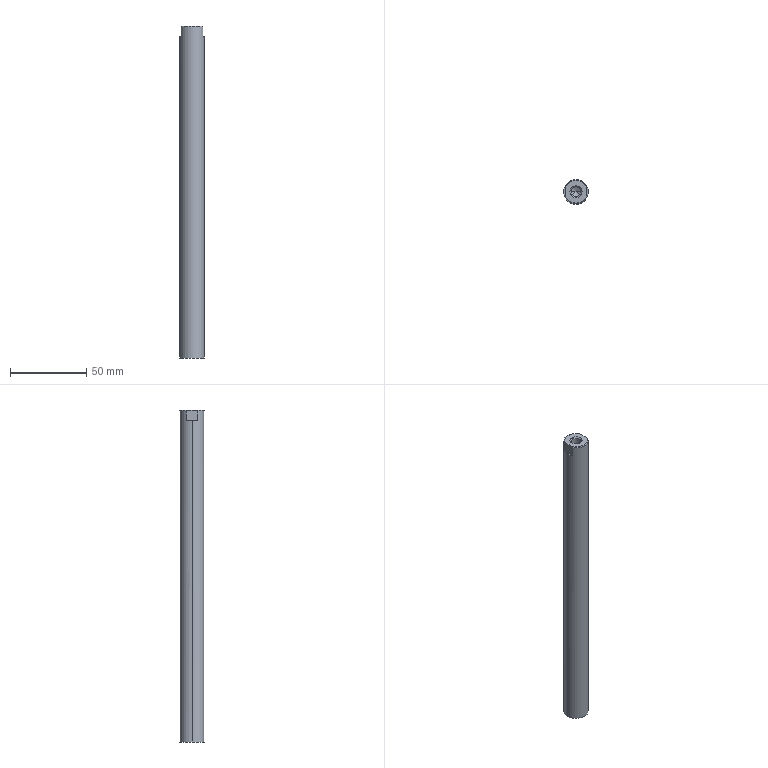Part | STEP file | A_CDQ2A32-200DC-F7NV(0) - Copy_Default | 1 solid | 16 faces | box 16 x 16 x 218 mm | volume 43283 mm3 | cone 6 | cylinder 4 | plane 4 | spline 2 | commonest cylinder face diameters 6.47 x2 16 x2
STEP:
#1=CARTESIAN_POINT('',(0.,0.,0.));
#2=DIRECTION('',(0.,0.,1.));
#3=DIRECTION('',(1.,0.,0.));
#4=AXIS2_PLACEMENT_3D('',#1,#2,#3);
#5=CARTESIAN_POINT('',(3.235,0.,16.235));
#6=VERTEX_POINT('',#5);
#7=CARTESIAN_POINT('',(4.,0.,17.));
#8=VERTEX_POINT('',#7);
#9=CARTESIAN_POINT('',(4.,0.,17.));
#10=DIRECTION('',(0.7071,0.,0.7071));
#11=VECTOR('',#10,1.);
#12=LINE('',#9,#11);
#13=CARTESIAN_POINT('',(0.,0.,17.));
#14=DIRECTION('',(0.,0.,1.));
#15=DIRECTION('',(1.,0.,0.));
#16=AXIS2_PLACEMENT_3D('',#13,#14,#15);
#17=CONICAL_SURFACE('',#16,4.,0.7854);
#18=CARTESIAN_POINT('',(6.283,0.));
#19=DIRECTION('',(0.,1.));
#20=VECTOR('',#19,1.);
#21=LINE('',#18,#20);
#22=(GEOMETRIC_REPRESENTATION_CONTEXT(2)PARAMETRIC_REPRESENTATION_CONTEXT()REPRESENTATION_CONTEXT('',''));
#23=DEFINITIONAL_REPRESENTATION('',(#21),#22);
#24=PCURVE('',#17,#23);
#25=CARTESIAN_POINT('',(0.,0.,17.));
#26=DIRECTION('',(0.,0.,1.));
#27=DIRECTION('',(1.,0.,0.));
#28=AXIS2_PLACEMENT_3D('',#25,#26,#27);
#29=CONICAL_SURFACE('',#28,4.,0.7854);
#30=CARTESIAN_POINT('',(0.,0.));
#31=DIRECTION('',(0.,1.));
#32=VECTOR('',#31,1.);
#33=LINE('',#30,#32);
#34=(GEOMETRIC_REPRESENTATION_CONTEXT(2)PARAMETRIC_REPRESENTATION_CONTEXT()REPRESENTATION_CONTEXT('',''));
#35=DEFINITIONAL_REPRESENTATION('',(#33),#34);
#36=PCURVE('',#29,#35);
#37=SURFACE_CURVE('',#12,(#24,#36),.PCURVE_S1.);
#38=EDGE_CURVE('',#6,#8,#37,.T.);
#39=ORIENTED_EDGE('',*,*,#38,.T.);
#40=CARTESIAN_POINT('',(-4.,0.,17.));
#41=VERTEX_POINT('',#40);
#42=CARTESIAN_POINT('',(0.,0.,17.));
#43=DIRECTION('',(0.,0.,1.));
#44=DIRECTION('',(1.,0.,0.));
#45=AXIS2_PLACEMENT_3D('',#42,#43,#44);
#46=CIRCLE('',#45,4.);
#47=CARTESIAN_POINT('',(0.,0.));
#48=DIRECTION('',(1.,0.));
#49=VECTOR('',#48,1.);
#50=LINE('',#47,#49);
#51=(GEOMETRIC_REPRESENTATION_CONTEXT(2)PARAMETRIC_REPRESENTATION_CONTEXT()REPRESENTATION_CONTEXT('',''));
#52=DEFINITIONAL_REPRESENTATION('',(#50),#51);
#53=PCURVE('',#17,#52);
#54=CARTESIAN_POINT('',(7.,-7.5,17.));
#55=DIRECTION('',(0.,0.,1.));
#56=DIRECTION('',(0.,1.,0.));
#57=AXIS2_PLACEMENT_3D('',#54,#55,#56);
#58=PLANE('',#57);
#59=CARTESIAN_POINT('',(7.5,7.));
#60=DIRECTION('',(0.,-1.));
#61=AXIS2_PLACEMENT_2D('',#59,#60);
#62=CIRCLE('',#61,4.);
#63=(GEOMETRIC_REPRESENTATION_CONTEXT(2)PARAMETRIC_REPRESENTATION_CONTEXT()REPRESENTATION_CONTEXT('',''));
#64=DEFINITIONAL_REPRESENTATION('',(#62),#63);
#65=PCURVE('',#58,#64);
#66=SURFACE_CURVE('',#46,(#53,#65),.PCURVE_S1.);
#67=EDGE_CURVE('',#41,#8,#66,.T.);
#68=ORIENTED_EDGE('',*,*,#67,.F.);
#69=CARTESIAN_POINT('',(-3.235,0.,16.235));
#70=VERTEX_POINT('',#69);
#71=CARTESIAN_POINT('',(-4.,0.,17.));
#72=DIRECTION('',(-0.7071,0.,0.7071));
#73=VECTOR('',#72,1.);
#74=LINE('',#71,#73);
#75=CARTESIAN_POINT('',(3.142,0.));
#76=DIRECTION('',(0.,1.));
#77=VECTOR('',#76,1.);
#78=LINE('',#75,#77);
#79=(GEOMETRIC_REPRESENTATION_CONTEXT(2)PARAMETRIC_REPRESENTATION_CONTEXT()REPRESENTATION_CONTEXT('',''));
#80=DEFINITIONAL_REPRESENTATION('',(#78),#79);
#81=PCURVE('',#17,#80);
#82=CARTESIAN_POINT('',(3.142,0.));
#83=DIRECTION('',(0.,1.));
#84=VECTOR('',#83,1.);
#85=LINE('',#82,#84);
#86=(GEOMETRIC_REPRESENTATION_CONTEXT(2)PARAMETRIC_REPRESENTATION_CONTEXT()REPRESENTATION_CONTEXT('',''));
#87=DEFINITIONAL_REPRESENTATION('',(#85),#86);
#88=PCURVE('',#29,#87);
#89=SURFACE_CURVE('',#74,(#81,#88),.PCURVE_S1.);
#90=EDGE_CURVE('',#70,#41,#89,.T.);
#91=ORIENTED_EDGE('',*,*,#90,.F.);
#92=CARTESIAN_POINT('',(0.,0.,16.235));
#93=DIRECTION('',(0.,0.,-1.));
#94=DIRECTION('',(0.,1.,0.));
#95=AXIS2_PLACEMENT_3D('',#92,#93,#94);
#96=CIRCLE('',#95,3.235);
#97=CARTESIAN_POINT('',(7.854,-0.765));
#98=DIRECTION('',(-1.,0.));
#99=VECTOR('',#98,1.);
#100=LINE('',#97,#99);
#101=(GEOMETRIC_REPRESENTATION_CONTEXT(2)PARAMETRIC_REPRESENTATION_CONTEXT()REPRESENTATION_CONTEXT('',''));
#102=DEFINITIONAL_REPRESENTATION('',(#100),#101);
#103=PCURVE('',#17,#102);
#104=CARTESIAN_POINT('',(0.,0.,3.5));
#105=DIRECTION('',(0.,0.,1.));
#106=DIRECTION('',(1.,0.,0.));
#107=AXIS2_PLACEMENT_3D('',#104,#105,#106);
#108=CYLINDRICAL_SURFACE('',#107,3.235);
#109=CARTESIAN_POINT('',(7.854,12.735));
#110=DIRECTION('',(-1.,0.));
#111=VECTOR('',#110,1.);
#112=LINE('',#109,#111);
#113=(GEOMETRIC_REPRESENTATION_CONTEXT(2)PARAMETRIC_REPRESENTATION_CONTEXT()REPRESENTATION_CONTEXT('',''));
#114=DEFINITIONAL_REPRESENTATION('',(#112),#113);
#115=PCURVE('',#108,#114);
#116=SURFACE_CURVE('',#96,(#103,#115),.PCURVE_S1.);
#117=EDGE_CURVE('',#6,#70,#116,.T.);
#118=ORIENTED_EDGE('',*,*,#117,.F.);
#119=EDGE_LOOP('',(#39,#68,#91,#118));
#120=FACE_BOUND('',#119,.F.);
#121=ADVANCED_FACE('',(#120),#17,.F.);
#122=CARTESIAN_POINT('',(3.235,0.,3.5));
#123=VERTEX_POINT('',#122);
#124=CARTESIAN_POINT('',(3.235,0.,3.5));
#125=DIRECTION('',(0.,0.,1.));
#126=VECTOR('',#125,1.);
#127=LINE('',#124,#126);
#128=CARTESIAN_POINT('',(6.283,0.));
#129=DIRECTION('',(0.,1.));
#130=VECTOR('',#129,1.);
#131=LINE('',#128,#130);
#132=(GEOMETRIC_REPRESENTATION_CONTEXT(2)PARAMETRIC_REPRESENTATION_CONTEXT()REPRESENTATION_CONTEXT('',''));
#133=DEFINITIONAL_REPRESENTATION('',(#131),#132);
#134=PCURVE('',#108,#133);
#135=CARTESIAN_POINT('',(0.,0.,3.5));
#136=DIRECTION('',(0.,0.,1.));
#137=DIRECTION('',(1.,0.,0.));
#138=AXIS2_PLACEMENT_3D('',#135,#136,#137);
#139=CYLINDRICAL_SURFACE('',#138,3.235);
#140=CARTESIAN_POINT('',(0.,0.));
#141=DIRECTION('',(0.,1.));
#142=VECTOR('',#141,1.);
#143=LINE('',#140,#142);
#144=(GEOMETRIC_REPRESENTATION_CONTEXT(2)PARAMETRIC_REPRESENTATION_CONTEXT()REPRESENTATION_CONTEXT('',''));
#145=DEFINITIONAL_REPRESENTATION('',(#143),#144);
#146=PCURVE('',#139,#145);
#147=SURFACE_CURVE('',#127,(#134,#146),.PCURVE_S1.);
#148=EDGE_CURVE('',#123,#6,#147,.T.);
#149=ORIENTED_EDGE('',*,*,#148,.T.);
#150=ORIENTED_EDGE('',*,*,#117,.T.);
#151=CARTESIAN_POINT('',(-3.235,0.,3.5));
#152=VERTEX_POINT('',#151);
#153=CARTESIAN_POINT('',(-3.235,0.,3.5));
#154=DIRECTION('',(0.,0.,1.));
#155=VECTOR('',#154,1.);
#156=LINE('',#153,#155);
#157=CARTESIAN_POINT('',(3.142,0.));
#158=DIRECTION('',(0.,1.));
#159=VECTOR('',#158,1.);
#160=LINE('',#157,#159);
#161=(GEOMETRIC_REPRESENTATION_CONTEXT(2)PARAMETRIC_REPRESENTATION_CONTEXT()REPRESENTATION_CONTEXT('',''));
#162=DEFINITIONAL_REPRESENTATION('',(#160),#161);
#163=PCURVE('',#108,#162);
#164=CARTESIAN_POINT('',(3.142,0.));
#165=DIRECTION('',(0.,1.));
#166=VECTOR('',#165,1.);
#167=LINE('',#164,#166);
#168=(GEOMETRIC_REPRESENTATION_CONTEXT(2)PARAMETRIC_REPRESENTATION_CONTEXT()REPRESENTATION_CONTEXT('',''));
#169=DEFINITIONAL_REPRESENTATION('',(#167),#168);
#170=PCURVE('',#139,#169);
#171=SURFACE_CURVE('',#156,(#163,#170),.PCURVE_S1.);
#172=EDGE_CURVE('',#152,#70,#171,.T.);
#173=ORIENTED_EDGE('',*,*,#172,.F.);
#174=CARTESIAN_POINT('',(0.,0.,3.5));
#175=DIRECTION('',(0.,0.,-1.));
#176=DIRECTION('',(0.,1.,0.));
#177=AXIS2_PLACEMENT_3D('',#174,#175,#176);
#178=CIRCLE('',#177,3.235);
#179=CARTESIAN_POINT('',(7.854,0.));
#180=DIRECTION('',(-1.,0.));
#181=VECTOR('',#180,1.);
#182=LINE('',#179,#181);
#183=(GEOMETRIC_REPRESENTATION_CONTEXT(2)PARAMETRIC_REPRESENTATION_CONTEXT()REPRESENTATION_CONTEXT('',''));
#184=DEFINITIONAL_REPRESENTATION('',(#182),#183);
#185=PCURVE('',#108,#184);
#186=CARTESIAN_POINT('',(0.,0.,3.5));
#187=DIRECTION('',(0.,0.,1.));
#188=DIRECTION('',(1.,0.,0.));
#189=AXIS2_PLACEMENT_3D('',#186,#187,#188);
#190=CONICAL_SURFACE('',#189,3.235,1.047);
#191=CARTESIAN_POINT('',(7.854,0.));
#192=DIRECTION('',(-1.,0.));
#193=VECTOR('',#192,1.);
#194=LINE('',#191,#193);
#195=(GEOMETRIC_REPRESENTATION_CONTEXT(2)PARAMETRIC_REPRESENTATION_CONTEXT()REPRESENTATION_CONTEXT('',''));
#196=DEFINITIONAL_REPRESENTATION('',(#194),#195);
#197=PCURVE('',#190,#196);
#198=SURFACE_CURVE('',#178,(#185,#197),.PCURVE_S1.);
#199=EDGE_CURVE('',#123,#152,#198,.T.);
#200=ORIENTED_EDGE('',*,*,#199,.F.);
#201=EDGE_LOOP('',(#149,#150,#173,#200));
#202=FACE_BOUND('',#201,.F.);
#203=ADVANCED_FACE('',(#202),#108,.F.);
#204=ORIENTED_EDGE('',*,*,#199,.T.);
#205=CARTESIAN_POINT('',(0.,0.,1.632));
#206=VERTEX_POINT('',#205);
#207=CARTESIAN_POINT('',(-3.235,0.,3.5));
#208=DIRECTION('',(-0.866,0.,0.5));
#209=VECTOR('',#208,1.);
#210=LINE('',#207,#209);
#211=CARTESIAN_POINT('',(3.142,0.));
#212=DIRECTION('',(0.,1.));
#213=VECTOR('',#212,1.);
#214=LINE('',#211,#213);
#215=(GEOMETRIC_REPRESENTATION_CONTEXT(2)PARAMETRIC_REPRESENTATION_CONTEXT()REPRESENTATION_CONTEXT('',''));
#216=DEFINITIONAL_REPRESENTATION('',(#214),#215);
#217=PCURVE('',#190,#216);
#218=CARTESIAN_POINT('',(0.,0.,3.5));
#219=DIRECTION('',(0.,0.,1.));
#220=DIRECTION('',(1.,0.,0.));
#221=AXIS2_PLACEMENT_3D('',#218,#219,#220);
#222=CONICAL_SURFACE('',#221,3.235,1.047);
#223=CARTESIAN_POINT('',(3.142,0.));
#224=DIRECTION('',(0.,1.));
#225=VECTOR('',#224,1.);
#226=LINE('',#223,#225);
#227=(GEOMETRIC_REPRESENTATION_CONTEXT(2)PARAMETRIC_REPRESENTATION_CONTEXT()REPRESENTATION_CONTEXT('',''));
#228=DEFINITIONAL_REPRESENTATION('',(#226),#227);
#229=PCURVE('',#222,#228);
#230=SURFACE_CURVE('',#210,(#217,#229),.PCURVE_S1.);
#231=EDGE_CURVE('',#206,#152,#230,.T.);
#232=ORIENTED_EDGE('',*,*,#231,.F.);
#233=CARTESIAN_POINT('',(3.235,0.,3.5));
#234=DIRECTION('',(0.866,0.,0.5));
#235=VECTOR('',#234,1.);
#236=LINE('',#233,#235);
#237=CARTESIAN_POINT('',(6.283,0.));
#238=DIRECTION('',(0.,1.));
#239=VECTOR('',#238,1.);
#240=LINE('',#237,#239);
#241=(GEOMETRIC_REPRESENTATION_CONTEXT(2)PARAMETRIC_REPRESENTATION_CONTEXT()REPRESENTATION_CONTEXT('',''));
#242=DEFINITIONAL_REPRESENTATION('',(#240),#241);
#243=PCURVE('',#190,#242);
#244=CARTESIAN_POINT('',(0.,0.));
#245=DIRECTION('',(0.,1.));
#246=VECTOR('',#245,1.);
#247=LINE('',#244,#246);
#248=(GEOMETRIC_REPRESENTATION_CONTEXT(2)PARAMETRIC_REPRESENTATION_CONTEXT()REPRESENTATION_CONTEXT('',''));
#249=DEFINITIONAL_REPRESENTATION('',(#247),#248);
#250=PCURVE('',#222,#249);
#251=SURFACE_CURVE('',#236,(#243,#250),.PCURVE_S1.);
#252=EDGE_CURVE('',#206,#123,#251,.T.);
#253=ORIENTED_EDGE('',*,*,#252,.T.);
#254=EDGE_LOOP('',(#204,#232,#253));
#255=FACE_BOUND('',#254,.F.);
#256=ADVANCED_FACE('',(#255),#190,.F.);
#257=CARTESIAN_POINT('',(8.,0.,-201.));
#258=VERTEX_POINT('',#257);
#259=CARTESIAN_POINT('',(-8.,0.,-201.));
#260=VERTEX_POINT('',#259);
#261=CARTESIAN_POINT('',(0.,0.,-201.));
#262=DIRECTION('',(0.,0.,1.));
#263=DIRECTION('',(1.,0.,0.));
#264=AXIS2_PLACEMENT_3D('',#261,#262,#263);
#265=CIRCLE('',#264,8.);
#266=CARTESIAN_POINT('',(0.,0.,16.5));
#267=DIRECTION('',(0.,0.,1.));
#268=DIRECTION('',(1.,0.,0.));
#269=AXIS2_PLACEMENT_3D('',#266,#267,#268);
#270=CYLINDRICAL_SURFACE('',#269,8.);
#271=CARTESIAN_POINT('',(0.,-217.5));
#272=DIRECTION('',(1.,0.));
#273=VECTOR('',#272,1.);
#274=LINE('',#271,#273);
#275=(GEOMETRIC_REPRESENTATION_CONTEXT(2)PARAMETRIC_REPRESENTATION_CONTEXT()REPRESENTATION_CONTEXT('',''));
#276=DEFINITIONAL_REPRESENTATION('',(#274),#275);
#277=PCURVE('',#270,#276);
#278=CARTESIAN_POINT('',(8.096,8.,-201.));
#279=DIRECTION('',(0.,0.,-1.));
#280=DIRECTION('',(0.,-1.,0.));
#281=AXIS2_PLACEMENT_3D('',#278,#279,#280);
#282=PLANE('',#281);
#283=CARTESIAN_POINT('',(8.,0.096));
#284=CARTESIAN_POINT('',(-5.856,0.096));
#285=CARTESIAN_POINT('',(1.072,12.096));
#286=CARTESIAN_POINT('',(8.,24.096));
#287=CARTESIAN_POINT('',(14.928,12.096));
#288=CARTESIAN_POINT('',(21.856,0.096));
#289=CARTESIAN_POINT('',(8.,0.096));
#290=(BOUNDED_CURVE()B_SPLINE_CURVE(2,(#283,#284,#285,#286,#287,#288,#289),.UNSPECIFIED.,.T.,.F.)B_SPLINE_CURVE_WITH_KNOTS((1,2,2,2,2,1),(-2.094,0.,2.094,4.189,6.283,8.378),.UNSPECIFIED.)CURVE()GEOMETRIC_REPRESENTATION_ITEM()RATIONAL_B_SPLINE_CURVE((1.,0.5,1.,0.5,1.,0.5,1.))REPRESENTATION_ITEM(''));
#291=(GEOMETRIC_REPRESENTATION_CONTEXT(2)PARAMETRIC_REPRESENTATION_CONTEXT()REPRESENTATION_CONTEXT('',''));
#292=DEFINITIONAL_REPRESENTATION('',(#290),#291);
#293=PCURVE('',#282,#292);
#294=SURFACE_CURVE('',#265,(#277,#293),.PCURVE_S1.);
#295=EDGE_CURVE('',#258,#260,#294,.T.);
#296=ORIENTED_EDGE('',*,*,#295,.T.);
#297=CARTESIAN_POINT('',(-8.,0.,10.));
#298=VERTEX_POINT('',#297);
#299=CARTESIAN_POINT('',(-8.,0.,16.5));
#300=DIRECTION('',(0.,0.,1.));
#301=VECTOR('',#300,1.);
#302=LINE('',#299,#301);
#303=CARTESIAN_POINT('',(3.142,0.));
#304=DIRECTION('',(0.,1.));
#305=VECTOR('',#304,1.);
#306=LINE('',#303,#305);
#307=(GEOMETRIC_REPRESENTATION_CONTEXT(2)PARAMETRIC_REPRESENTATION_CONTEXT()REPRESENTATION_CONTEXT('',''));
#308=DEFINITIONAL_REPRESENTATION('',(#306),#307);
#309=PCURVE('',#270,#308);
#310=CARTESIAN_POINT('',(0.,0.,16.5));
#311=DIRECTION('',(0.,0.,1.));
#312=DIRECTION('',(1.,0.,0.));
#313=AXIS2_PLACEMENT_3D('',#310,#311,#312);
#314=CYLINDRICAL_SURFACE('',#313,8.);
#315=CARTESIAN_POINT('',(3.142,0.));
#316=DIRECTION('',(0.,1.));
#317=VECTOR('',#316,1.);
#318=LINE('',#315,#317);
#319=(GEOMETRIC_REPRESENTATION_CONTEXT(2)PARAMETRIC_REPRESENTATION_CONTEXT()REPRESENTATION_CONTEXT('',''));
#320=DEFINITIONAL_REPRESENTATION('',(#318),#319);
#321=PCURVE('',#314,#320);
#322=SURFACE_CURVE('',#302,(#309,#321),.PCURVE_S1.);
#323=EDGE_CURVE('',#260,#298,#322,.T.);
#324=ORIENTED_EDGE('',*,*,#323,.T.);
#325=CARTESIAN_POINT('',(-7.,3.873,10.));
#326=VERTEX_POINT('',#325);
#327=CARTESIAN_POINT('',(0.,0.,10.));
#328=DIRECTION('',(0.,0.,-1.));
#329=DIRECTION('',(1.,0.,0.));
#330=AXIS2_PLACEMENT_3D('',#327,#328,#329);
#331=CIRCLE('',#330,8.);
#332=CARTESIAN_POINT('',(6.283,-6.5));
#333=DIRECTION('',(-1.,0.));
#334=VECTOR('',#333,1.);
#335=LINE('',#332,#334);
#336=(GEOMETRIC_REPRESENTATION_CONTEXT(2)PARAMETRIC_REPRESENTATION_CONTEXT()REPRESENTATION_CONTEXT('',''));
#337=DEFINITIONAL_REPRESENTATION('',(#335),#336);
#338=PCURVE('',#270,#337);
#339=CARTESIAN_POINT('',(-8.13,-3.919,10.));
#340=CARTESIAN_POINT('',(-8.13,3.919,10.));
#341=CARTESIAN_POINT('',(-8.01,-3.919,10.));
#342=CARTESIAN_POINT('',(-8.01,3.919,10.));
#343=CARTESIAN_POINT('',(-8.,-3.919,10.));
#344=CARTESIAN_POINT('',(-8.,3.919,10.));
#345=CARTESIAN_POINT('',(-7.,-3.919,10.));
#346=CARTESIAN_POINT('',(-7.,3.919,10.));
#347=B_SPLINE_SURFACE_WITH_KNOTS('',1,1,((#339,#340),(#341,#342),(#343,#344),(#345,#346)),.UNSPECIFIED.,.F.,.F.,.F.,(2,1,1,2),(2,2),(-0.1295,-0.01,0.,1.),(0.,1.),.UNSPECIFIED.);
#348=CARTESIAN_POINT('',(0.,0.5));
#349=CARTESIAN_POINT('',(-0.000000185,0.5078));
#350=CARTESIAN_POINT('',(0.001407,0.5234));
#351=CARTESIAN_POINT('',(0.007738,0.5469));
#352=CARTESIAN_POINT('',(0.01829,0.5703));
#353=CARTESIAN_POINT('',(0.03305,0.5936));
#354=CARTESIAN_POINT('',(0.05201,0.617));
#355=CARTESIAN_POINT('',(0.07517,0.6402));
#356=CARTESIAN_POINT('',(0.1025,0.6634));
#357=CARTESIAN_POINT('',(0.134,0.6865));
#358=CARTESIAN_POINT('',(0.1697,0.7095));
#359=CARTESIAN_POINT('',(0.2095,0.7324));
#360=CARTESIAN_POINT('',(0.2534,0.7552));
#361=CARTESIAN_POINT('',(0.3013,0.7778));
#362=CARTESIAN_POINT('',(0.3534,0.8003));
#363=CARTESIAN_POINT('',(0.4095,0.8226));
#364=CARTESIAN_POINT('',(0.4696,0.8448));
#365=CARTESIAN_POINT('',(0.5336,0.8667));
#366=CARTESIAN_POINT('',(0.6016,0.8885));
#367=CARTESIAN_POINT('',(0.6735,0.9101));
#368=CARTESIAN_POINT('',(0.7493,0.9314));
#369=CARTESIAN_POINT('',(0.8289,0.9526));
#370=CARTESIAN_POINT('',(0.9123,0.9735));
#371=CARTESIAN_POINT('',(0.9703,0.9872));
#372=CARTESIAN_POINT('',(1.,0.9941));
#373=B_SPLINE_CURVE_WITH_KNOTS('',3,(#348,#349,#350,#351,#352,#353,#354,#355,#356,#357,#358,#359,#360,#361,#362,#363,#364,#365,#366,#367,#368,#369,#370,#371,#372),.UNSPECIFIED.,.F.,.F.,(4,1,1,1,1,1,1,1,1,1,1,1,1,1,1,1,1,1,1,1,1,1,4),(3.142,3.165,3.188,3.211,3.233,3.256,3.279,3.302,3.325,3.348,3.371,3.394,3.417,3.44,3.463,3.486,3.509,3.532,3.555,3.578,3.601,3.624,3.647),.QUASI_UNIFORM_KNOTS.);
#374=(GEOMETRIC_REPRESENTATION_CONTEXT(2)PARAMETRIC_REPRESENTATION_CONTEXT()REPRESENTATION_CONTEXT('',''));
#375=DEFINITIONAL_REPRESENTATION('',(#373),#374);
#376=PCURVE('',#347,#375);
#377=SURFACE_CURVE('',#331,(#338,#376),.PCURVE_S1.);
#378=EDGE_CURVE('',#298,#326,#377,.T.);
#379=ORIENTED_EDGE('',*,*,#378,.T.);
#380=CARTESIAN_POINT('',(-7.,3.873,16.5));
#381=VERTEX_POINT('',#380);
#382=CARTESIAN_POINT('',(-7.,3.873,17.));
#383=DIRECTION('',(0.,0.,-1.));
#384=VECTOR('',#383,1.);
#385=LINE('',#382,#384);
#386=CARTESIAN_POINT('',(2.636,0.5));
#387=DIRECTION('',(0.,-1.));
#388=VECTOR('',#387,1.);
#389=LINE('',#386,#388);
#390=(GEOMETRIC_REPRESENTATION_CONTEXT(2)PARAMETRIC_REPRESENTATION_CONTEXT()REPRESENTATION_CONTEXT('',''));
#391=DEFINITIONAL_REPRESENTATION('',(#389),#390);
#392=PCURVE('',#270,#391);
#393=CARTESIAN_POINT('',(-7.,-3.873,17.));
#394=DIRECTION('',(-1.,0.,0.));
#395=DIRECTION('',(0.,1.,0.));
#396=AXIS2_PLACEMENT_3D('',#393,#394,#395);
#397=PLANE('',#396);
#398=CARTESIAN_POINT('',(7.746,0.));
#399=DIRECTION('',(0.,1.));
#400=VECTOR('',#399,1.);
#401=LINE('',#398,#400);
#402=(GEOMETRIC_REPRESENTATION_CONTEXT(2)PARAMETRIC_REPRESENTATION_CONTEXT()REPRESENTATION_CONTEXT('',''));
#403=DEFINITIONAL_REPRESENTATION('',(#401),#402);
#404=PCURVE('',#397,#403);
#405=SURFACE_CURVE('',#385,(#392,#404),.PCURVE_S1.);
#406=EDGE_CURVE('',#381,#326,#405,.T.);
#407=ORIENTED_EDGE('',*,*,#406,.F.);
#408=CARTESIAN_POINT('',(7.,3.873,16.5));
#409=VERTEX_POINT('',#408);
#410=CARTESIAN_POINT('',(0.,0.,16.5));
#411=DIRECTION('',(0.,0.,1.));
#412=DIRECTION('',(0.,1.,0.));
#413=AXIS2_PLACEMENT_3D('',#410,#411,#412);
#414=CIRCLE('',#413,8.);
#415=CARTESIAN_POINT('',(-4.712,0.));
#416=DIRECTION('',(1.,0.));
#417=VECTOR('',#416,1.);
#418=LINE('',#415,#417);
#419=(GEOMETRIC_REPRESENTATION_CONTEXT(2)PARAMETRIC_REPRESENTATION_CONTEXT()REPRESENTATION_CONTEXT('',''));
#420=DEFINITIONAL_REPRESENTATION('',(#418),#419);
#421=PCURVE('',#270,#420);
#422=CARTESIAN_POINT('',(0.,0.,17.));
#423=DIRECTION('',(0.,0.,-1.));
#424=DIRECTION('',(-1.,0.,0.));
#425=AXIS2_PLACEMENT_3D('',#422,#423,#424);
#426=CONICAL_SURFACE('',#425,7.5,0.7854);
#427=CARTESIAN_POINT('',(7.854,0.5));
#428=DIRECTION('',(-1.,0.));
#429=VECTOR('',#428,1.);
#430=LINE('',#427,#429);
#431=(GEOMETRIC_REPRESENTATION_CONTEXT(2)PARAMETRIC_REPRESENTATION_CONTEXT()REPRESENTATION_CONTEXT('',''));
#432=DEFINITIONAL_REPRESENTATION('',(#430),#431);
#433=PCURVE('',#426,#432);
#434=SURFACE_CURVE('',#414,(#421,#433),.PCURVE_S1.);
#435=EDGE_CURVE('',#409,#381,#434,.T.);
#436=ORIENTED_EDGE('',*,*,#435,.F.);
#437=CARTESIAN_POINT('',(7.,3.873,10.));
#438=VERTEX_POINT('',#437);
#439=CARTESIAN_POINT('',(7.,3.873,17.));
#440=DIRECTION('',(0.,0.,1.));
#441=VECTOR('',#440,1.);
#442=LINE('',#439,#441);
#443=CARTESIAN_POINT('',(0.5054,0.5));
#444=DIRECTION('',(0.,1.));
#445=VECTOR('',#444,1.);
#446=LINE('',#443,#445);
#447=(GEOMETRIC_REPRESENTATION_CONTEXT(2)PARAMETRIC_REPRESENTATION_CONTEXT()REPRESENTATION_CONTEXT('',''));
#448=DEFINITIONAL_REPRESENTATION('',(#446),#447);
#449=PCURVE('',#270,#448);
#450=CARTESIAN_POINT('',(7.,3.873,17.));
#451=DIRECTION('',(1.,0.,0.));
#452=DIRECTION('',(0.,-1.,0.));
#453=AXIS2_PLACEMENT_3D('',#450,#451,#452);
#454=PLANE('',#453);
#455=CARTESIAN_POINT('',(0.,0.));
#456=DIRECTION('',(0.,-1.));
#457=VECTOR('',#456,1.);
#458=LINE('',#455,#457);
#459=(GEOMETRIC_REPRESENTATION_CONTEXT(2)PARAMETRIC_REPRESENTATION_CONTEXT()REPRESENTATION_CONTEXT('',''));
#460=DEFINITIONAL_REPRESENTATION('',(#458),#459);
#461=PCURVE('',#454,#460);
#462=SURFACE_CURVE('',#442,(#449,#461),.PCURVE_S1.);
#463=EDGE_CURVE('',#438,#409,#462,.T.);
#464=ORIENTED_EDGE('',*,*,#463,.F.);
#465=CARTESIAN_POINT('',(8.,0.,10.));
#466=VERTEX_POINT('',#465);
#467=CARTESIAN_POINT('',(0.,0.,10.));
#468=DIRECTION('',(0.,0.,-1.));
#469=DIRECTION('',(1.,0.,0.));
#470=AXIS2_PLACEMENT_3D('',#467,#468,#469);
#471=CIRCLE('',#470,8.);
#472=CARTESIAN_POINT('',(6.283,-6.5));
#473=DIRECTION('',(-1.,0.));
#474=VECTOR('',#473,1.);
#475=LINE('',#472,#474);
#476=(GEOMETRIC_REPRESENTATION_CONTEXT(2)PARAMETRIC_REPRESENTATION_CONTEXT()REPRESENTATION_CONTEXT('',''));
#477=DEFINITIONAL_REPRESENTATION('',(#475),#476);
#478=PCURVE('',#270,#477);
#479=CARTESIAN_POINT('',(7.,-3.919,10.));
#480=CARTESIAN_POINT('',(7.,3.919,10.));
#481=CARTESIAN_POINT('',(8.,-3.919,10.));
#482=CARTESIAN_POINT('',(8.,3.919,10.));
#483=CARTESIAN_POINT('',(8.01,-3.919,10.));
#484=CARTESIAN_POINT('',(8.01,3.919,10.));
#485=CARTESIAN_POINT('',(8.13,-3.919,10.));
#486=CARTESIAN_POINT('',(8.13,3.919,10.));
#487=B_SPLINE_SURFACE_WITH_KNOTS('',1,1,((#479,#480),(#481,#482),(#483,#484),(#485,#486)),.UNSPECIFIED.,.F.,.F.,.F.,(2,1,1,2),(2,2),(0.,1.,1.01,1.13),(0.,1.),.UNSPECIFIED.);
#488=CARTESIAN_POINT('',(0.,0.9941));
#489=CARTESIAN_POINT('',(0.02966,0.9872));
#490=CARTESIAN_POINT('',(0.08773,0.9735));
#491=CARTESIAN_POINT('',(0.1711,0.9526));
#492=CARTESIAN_POINT('',(0.2507,0.9314));
#493=CARTESIAN_POINT('',(0.3265,0.9101));
#494=CARTESIAN_POINT('',(0.3984,0.8885));
#495=CARTESIAN_POINT('',(0.4664,0.8667));
#496=CARTESIAN_POINT('',(0.5304,0.8448));
#497=CARTESIAN_POINT('',(0.5905,0.8226));
#498=CARTESIAN_POINT('',(0.6466,0.8003));
#499=CARTESIAN_POINT('',(0.6987,0.7778));
#500=CARTESIAN_POINT('',(0.7466,0.7552));
#501=CARTESIAN_POINT('',(0.7905,0.7324));
#502=CARTESIAN_POINT('',(0.8303,0.7095));
#503=CARTESIAN_POINT('',(0.866,0.6865));
#504=CARTESIAN_POINT('',(0.8975,0.6634));
#505=CARTESIAN_POINT('',(0.9248,0.6402));
#506=CARTESIAN_POINT('',(0.948,0.617));
#507=CARTESIAN_POINT('',(0.967,0.5936));
#508=CARTESIAN_POINT('',(0.9817,0.5703));
#509=CARTESIAN_POINT('',(0.9923,0.5469));
#510=CARTESIAN_POINT('',(0.9986,0.5234));
#511=CARTESIAN_POINT('',(1.,0.5078));
#512=CARTESIAN_POINT('',(1.,0.5));
#513=B_SPLINE_CURVE_WITH_KNOTS('',3,(#488,#489,#490,#491,#492,#493,#494,#495,#496,#497,#498,#499,#500,#501,#502,#503,#504,#505,#506,#507,#508,#509,#510,#511,#512),.UNSPECIFIED.,.F.,.F.,(4,1,1,1,1,1,1,1,1,1,1,1,1,1,1,1,1,1,1,1,1,1,4),(5.778,5.801,5.824,5.847,5.87,5.893,5.916,5.939,5.962,5.985,6.008,6.031,6.053,6.076,6.099,6.122,6.145,6.168,6.191,6.214,6.237,6.26,6.283),.QUASI_UNIFORM_KNOTS.);
#514=(GEOMETRIC_REPRESENTATION_CONTEXT(2)PARAMETRIC_REPRESENTATION_CONTEXT()REPRESENTATION_CONTEXT('',''));
#515=DEFINITIONAL_REPRESENTATION('',(#513),#514);
#516=PCURVE('',#487,#515);
#517=SURFACE_CURVE('',#471,(#478,#516),.PCURVE_S1.);
#518=EDGE_CURVE('',#438,#466,#517,.T.);
#519=ORIENTED_EDGE('',*,*,#518,.T.);
#520=CARTESIAN_POINT('',(8.,0.,16.5));
#521=DIRECTION('',(0.,0.,1.));
#522=VECTOR('',#521,1.);
#523=LINE('',#520,#522);
#524=CARTESIAN_POINT('',(0.,0.));
#525=DIRECTION('',(0.,1.));
#526=VECTOR('',#525,1.);
#527=LINE('',#524,#526);
#528=(GEOMETRIC_REPRESENTATION_CONTEXT(2)PARAMETRIC_REPRESENTATION_CONTEXT()REPRESENTATION_CONTEXT('',''));
#529=DEFINITIONAL_REPRESENTATION('',(#527),#528);
#530=PCURVE('',#270,#529);
#531=CARTESIAN_POINT('',(6.283,0.));
#532=DIRECTION('',(0.,1.));
#533=VECTOR('',#532,1.);
#534=LINE('',#531,#533);
#535=(GEOMETRIC_REPRESENTATION_CONTEXT(2)PARAMETRIC_REPRESENTATION_CONTEXT()REPRESENTATION_CONTEXT('',''));
#536=DEFINITIONAL_REPRESENTATION('',(#534),#535);
#537=PCURVE('',#314,#536);
#538=SURFACE_CURVE('',#523,(#530,#537),.PCURVE_S1.);
#539=EDGE_CURVE('',#258,#466,#538,.T.);
#540=ORIENTED_EDGE('',*,*,#539,.F.);
#541=EDGE_LOOP('',(#296,#324,#379,#407,#436,#464,#519,#540));
#542=FACE_BOUND('',#541,.T.);
#543=ADVANCED_FACE('',(#542),#270,.T.);
#544=CARTESIAN_POINT('',(0.,0.,17.));
#545=DIRECTION('',(0.,0.,1.));
#546=DIRECTION('',(1.,0.,0.));
#547=AXIS2_PLACEMENT_3D('',#544,#545,#546);
#548=CIRCLE('',#547,4.);
#549=CARTESIAN_POINT('',(0.,0.));
#550=DIRECTION('',(1.,0.));
#551=VECTOR('',#550,1.);
#552=LINE('',#549,#551);
#553=(GEOMETRIC_REPRESENTATION_CONTEXT(2)PARAMETRIC_REPRESENTATION_CONTEXT()REPRESENTATION_CONTEXT('',''));
#554=DEFINITIONAL_REPRESENTATION('',(#552),#553);
#555=PCURVE('',#29,#554);
#556=CARTESIAN_POINT('',(7.5,7.));
#557=DIRECTION('',(0.,-1.));
#558=AXIS2_PLACEMENT_2D('',#556,#557);
#559=CIRCLE('',#558,4.);
#560=(GEOMETRIC_REPRESENTATION_CONTEXT(2)PARAMETRIC_REPRESENTATION_CONTEXT()REPRESENTATION_CONTEXT('',''));
#561=DEFINITIONAL_REPRESENTATION('',(#559),#560);
#562=PCURVE('',#58,#561);
#563=SURFACE_CURVE('',#548,(#555,#562),.PCURVE_S1.);
#564=EDGE_CURVE('',#8,#41,#563,.T.);
#565=ORIENTED_EDGE('',*,*,#564,.F.);
#566=ORIENTED_EDGE('',*,*,#38,.F.);
#567=CARTESIAN_POINT('',(0.,0.,16.235));
#568=DIRECTION('',(0.,0.,-1.));
#569=DIRECTION('',(0.,1.,0.));
#570=AXIS2_PLACEMENT_3D('',#567,#568,#569);
#571=CIRCLE('',#570,3.235);
#572=CARTESIAN_POINT('',(7.854,-0.765));
#573=DIRECTION('',(-1.,0.));
#574=VECTOR('',#573,1.);
#575=LINE('',#572,#574);
#576=(GEOMETRIC_REPRESENTATION_CONTEXT(2)PARAMETRIC_REPRESENTATION_CONTEXT()REPRESENTATION_CONTEXT('',''));
#577=DEFINITIONAL_REPRESENTATION('',(#575),#576);
#578=PCURVE('',#29,#577);
#579=CARTESIAN_POINT('',(7.854,12.735));
#580=DIRECTION('',(-1.,0.));
#581=VECTOR('',#580,1.);
#582=LINE('',#579,#581);
#583=(GEOMETRIC_REPRESENTATION_CONTEXT(2)PARAMETRIC_REPRESENTATION_CONTEXT()REPRESENTATION_CONTEXT('',''));
#584=DEFINITIONAL_REPRESENTATION('',(#582),#583);
#585=PCURVE('',#139,#584);
#586=SURFACE_CURVE('',#571,(#578,#585),.PCURVE_S1.);
#587=EDGE_CURVE('',#70,#6,#586,.T.);
#588=ORIENTED_EDGE('',*,*,#587,.F.);
#589=ORIENTED_EDGE('',*,*,#90,.T.);
#590=EDGE_LOOP('',(#565,#566,#588,#589));
#591=FACE_BOUND('',#590,.F.);
#592=ADVANCED_FACE('',(#591),#29,.F.);
#593=ORIENTED_EDGE('',*,*,#587,.T.);
#594=ORIENTED_EDGE('',*,*,#148,.F.);
#595=CARTESIAN_POINT('',(0.,0.,3.5));
#596=DIRECTION('',(0.,0.,-1.));
#597=DIRECTION('',(0.,1.,0.));
#598=AXIS2_PLACEMENT_3D('',#595,#596,#597);
#599=CIRCLE('',#598,3.235);
#600=CARTESIAN_POINT('',(7.854,0.));
#601=DIRECTION('',(-1.,0.));
#602=VECTOR('',#601,1.);
#603=LINE('',#600,#602);
#604=(GEOMETRIC_REPRESENTATION_CONTEXT(2)PARAMETRIC_REPRESENTATION_CONTEXT()REPRESENTATION_CONTEXT('',''));
#605=DEFINITIONAL_REPRESENTATION('',(#603),#604);
#606=PCURVE('',#139,#605);
#607=CARTESIAN_POINT('',(7.854,0.));
#608=DIRECTION('',(-1.,0.));
#609=VECTOR('',#608,1.);
#610=LINE('',#607,#609);
#611=(GEOMETRIC_REPRESENTATION_CONTEXT(2)PARAMETRIC_REPRESENTATION_CONTEXT()REPRESENTATION_CONTEXT('',''));
#612=DEFINITIONAL_REPRESENTATION('',(#610),#611);
#613=PCURVE('',#222,#612);
#614=SURFACE_CURVE('',#599,(#606,#613),.PCURVE_S1.);
#615=EDGE_CURVE('',#152,#123,#614,.T.);
#616=ORIENTED_EDGE('',*,*,#615,.F.);
#617=ORIENTED_EDGE('',*,*,#172,.T.);
#618=EDGE_LOOP('',(#593,#594,#616,#617));
#619=FACE_BOUND('',#618,.F.);
#620=ADVANCED_FACE('',(#619),#139,.F.);
#621=ORIENTED_EDGE('',*,*,#564,.F.);
#622=ORIENTED_EDGE('',*,*,#67,.F.);
#623=EDGE_LOOP('',(#621,#622));
#624=FACE_BOUND('',#623,.T.);
#625=CARTESIAN_POINT('',(7.,-2.693,17.));
#626=VERTEX_POINT('',#625);
#627=CARTESIAN_POINT('',(7.,2.693,17.));
#628=VERTEX_POINT('',#627);
#629=CARTESIAN_POINT('',(7.,0.,17.));
#630=DIRECTION('',(0.,1.,0.));
#631=VECTOR('',#630,1.);
#632=LINE('',#629,#631);
#633=CARTESIAN_POINT('',(7.5,0.));
#634=DIRECTION('',(1.,0.));
#635=VECTOR('',#634,1.);
#636=LINE('',#633,#635);
#637=(GEOMETRIC_REPRESENTATION_CONTEXT(2)PARAMETRIC_REPRESENTATION_CONTEXT()REPRESENTATION_CONTEXT('',''));
#638=DEFINITIONAL_REPRESENTATION('',(#636),#637);
#639=PCURVE('',#58,#638);
#640=CARTESIAN_POINT('',(3.873,0.));
#641=DIRECTION('',(-1.,0.));
#642=VECTOR('',#641,1.);
#643=LINE('',#640,#642);
#644=(GEOMETRIC_REPRESENTATION_CONTEXT(2)PARAMETRIC_REPRESENTATION_CONTEXT()REPRESENTATION_CONTEXT('',''));
#645=DEFINITIONAL_REPRESENTATION('',(#643),#644);
#646=PCURVE('',#454,#645);
#647=SURFACE_CURVE('',#632,(#639,#646),.PCURVE_S1.);
#648=EDGE_CURVE('',#626,#628,#647,.T.);
#649=ORIENTED_EDGE('',*,*,#648,.T.);
#650=CARTESIAN_POINT('',(-7.,2.693,17.));
#651=VERTEX_POINT('',#650);
#652=CARTESIAN_POINT('',(0.,0.,17.));
#653=DIRECTION('',(0.,0.,1.));
#654=DIRECTION('',(-1.,0.,0.));
#655=AXIS2_PLACEMENT_3D('',#652,#653,#654);
#656=CIRCLE('',#655,7.5);
#657=CARTESIAN_POINT('',(7.5,7.));
#658=DIRECTION('',(0.,1.));
#659=AXIS2_PLACEMENT_2D('',#657,#658);
#660=CIRCLE('',#659,7.5);
#661=(GEOMETRIC_REPRESENTATION_CONTEXT(2)PARAMETRIC_REPRESENTATION_CONTEXT()REPRESENTATION_CONTEXT('',''));
#662=DEFINITIONAL_REPRESENTATION('',(#660),#661);
#663=PCURVE('',#58,#662);
#664=CARTESIAN_POINT('',(6.283,0.));
#665=DIRECTION('',(-1.,0.));
#666=VECTOR('',#665,1.);
#667=LINE('',#664,#666);
#668=(GEOMETRIC_REPRESENTATION_CONTEXT(2)PARAMETRIC_REPRESENTATION_CONTEXT()REPRESENTATION_CONTEXT('',''));
#669=DEFINITIONAL_REPRESENTATION('',(#667),#668);
#670=PCURVE('',#426,#669);
#671=SURFACE_CURVE('',#656,(#663,#670),.PCURVE_S1.);
#672=EDGE_CURVE('',#628,#651,#671,.T.);
#673=ORIENTED_EDGE('',*,*,#672,.T.);
#674=CARTESIAN_POINT('',(-7.,-2.693,17.));
#675=VERTEX_POINT('',#674);
#676=CARTESIAN_POINT('',(-7.,0.,17.));
#677=DIRECTION('',(0.,-1.,0.));
#678=VECTOR('',#677,1.);
#679=LINE('',#676,#678);
#680=CARTESIAN_POINT('',(7.5,14.));
#681=DIRECTION('',(-1.,0.));
#682=VECTOR('',#681,1.);
#683=LINE('',#680,#682);
#684=(GEOMETRIC_REPRESENTATION_CONTEXT(2)PARAMETRIC_REPRESENTATION_CONTEXT()REPRESENTATION_CONTEXT('',''));
#685=DEFINITIONAL_REPRESENTATION('',(#683),#684);
#686=PCURVE('',#58,#685);
#687=CARTESIAN_POINT('',(3.873,0.));
#688=DIRECTION('',(-1.,0.));
#689=VECTOR('',#688,1.);
#690=LINE('',#687,#689);
#691=(GEOMETRIC_REPRESENTATION_CONTEXT(2)PARAMETRIC_REPRESENTATION_CONTEXT()REPRESENTATION_CONTEXT('',''));
#692=DEFINITIONAL_REPRESENTATION('',(#690),#691);
#693=PCURVE('',#397,#692);
#694=SURFACE_CURVE('',#679,(#686,#693),.PCURVE_S1.);
#695=EDGE_CURVE('',#651,#675,#694,.T.);
#696=ORIENTED_EDGE('',*,*,#695,.T.);
#697=CARTESIAN_POINT('',(0.,0.,17.));
#698=DIRECTION('',(0.,0.,1.));
#699=DIRECTION('',(-1.,0.,0.));
#700=AXIS2_PLACEMENT_3D('',#697,#698,#699);
#701=CIRCLE('',#700,7.5);
#702=CARTESIAN_POINT('',(7.5,7.));
#703=DIRECTION('',(0.,1.));
#704=AXIS2_PLACEMENT_2D('',#702,#703);
#705=CIRCLE('',#704,7.5);
#706=(GEOMETRIC_REPRESENTATION_CONTEXT(2)PARAMETRIC_REPRESENTATION_CONTEXT()REPRESENTATION_CONTEXT('',''));
#707=DEFINITIONAL_REPRESENTATION('',(#705),#706);
#708=PCURVE('',#58,#707);
#709=CARTESIAN_POINT('',(0.,0.,17.));
#710=DIRECTION('',(0.,0.,-1.));
#711=DIRECTION('',(-1.,0.,0.));
#712=AXIS2_PLACEMENT_3D('',#709,#710,#711);
#713=CONICAL_SURFACE('',#712,7.5,0.7854);
#714=CARTESIAN_POINT('',(6.283,0.));
#715=DIRECTION('',(-1.,0.));
#716=VECTOR('',#715,1.);
#717=LINE('',#714,#716);
#718=(GEOMETRIC_REPRESENTATION_CONTEXT(2)PARAMETRIC_REPRESENTATION_CONTEXT()REPRESENTATION_CONTEXT('',''));
#719=DEFINITIONAL_REPRESENTATION('',(#717),#718);
#720=PCURVE('',#713,#719);
#721=SURFACE_CURVE('',#701,(#708,#720),.PCURVE_S1.);
#722=EDGE_CURVE('',#675,#626,#721,.T.);
#723=ORIENTED_EDGE('',*,*,#722,.T.);
#724=EDGE_LOOP('',(#649,#673,#696,#723));
#725=FACE_BOUND('',#724,.T.);
#726=ADVANCED_FACE('',(#624,#725),#58,.T.);
#727=ORIENTED_EDGE('',*,*,#615,.T.);
#728=ORIENTED_EDGE('',*,*,#252,.F.);
#729=ORIENTED_EDGE('',*,*,#231,.T.);
#730=EDGE_LOOP('',(#727,#728,#729));
#731=FACE_BOUND('',#730,.F.);
#732=ADVANCED_FACE('',(#731),#222,.F.);
#733=CARTESIAN_POINT('',(-7.,3.873,16.5));
#734=CARTESIAN_POINT('',(-7.,3.488,16.686));
#735=CARTESIAN_POINT('',(-7.,3.095,16.855));
#736=CARTESIAN_POINT('',(-7.,2.693,17.));
#737=B_SPLINE_CURVE_WITH_KNOTS('',3,(#733,#734,#735,#736),.UNSPECIFIED.,.F.,.F.,(4,4),(0.,0.001282),.PIECEWISE_BEZIER_KNOTS.);
#738=CARTESIAN_POINT('',(0.5054,0.5));
#739=CARTESIAN_POINT('',(0.5034,0.4915));
#740=CARTESIAN_POINT('',(0.4996,0.4747));
#741=CARTESIAN_POINT('',(0.4938,0.4496));
#742=CARTESIAN_POINT('',(0.4879,0.4247));
#743=CARTESIAN_POINT('',(0.482,0.4001));
#744=CARTESIAN_POINT('',(0.4761,0.3756));
#745=CARTESIAN_POINT('',(0.4701,0.3515));
#746=CARTESIAN_POINT('',(0.464,0.3275));
#747=CARTESIAN_POINT('',(0.4579,0.3039));
#748=CARTESIAN_POINT('',(0.4518,0.2804));
#749=CARTESIAN_POINT('',(0.4456,0.2572));
#750=CARTESIAN_POINT('',(0.4393,0.2343));
#751=CARTESIAN_POINT('',(0.433,0.2116));
#752=CARTESIAN_POINT('',(0.4267,0.1892));
#753=CARTESIAN_POINT('',(0.4203,0.1671));
#754=CARTESIAN_POINT('',(0.4138,0.1452));
#755=CARTESIAN_POINT('',(0.4073,0.1236));
#756=CARTESIAN_POINT('',(0.4007,0.1023));
#757=CARTESIAN_POINT('',(0.3941,0.08121));
#758=CARTESIAN_POINT('',(0.3875,0.06046));
#759=CARTESIAN_POINT('',(0.3808,0.03999));
#760=CARTESIAN_POINT('',(0.374,0.01982));
#761=CARTESIAN_POINT('',(0.3695,0.006573));
#762=CARTESIAN_POINT('',(0.3672,0.));
#763=B_SPLINE_CURVE_WITH_KNOTS('',3,(#738,#739,#740,#741,#742,#743,#744,#745,#746,#747,#748,#749,#750,#751,#752,#753,#754,#755,#756,#757,#758,#759,#760,#761,#762),.UNSPECIFIED.,.F.,.F.,(4,1,1,1,1,1,1,1,1,1,1,1,1,1,1,1,1,1,1,1,1,1,4),(0.,0.00005827,0.0001165,0.0001748,0.0002331,0.0002913,0.0003496,0.0004079,0.0004662,0.0005244,0.0005827,0.000641,0.0006992,0.0007575,0.0008158,0.000874,0.0009323,0.0009906,0.001049,0.001107,0.001165,0.001224,0.001282),.QUASI_UNIFORM_KNOTS.);
#764=(GEOMETRIC_REPRESENTATION_CONTEXT(2)PARAMETRIC_REPRESENTATION_CONTEXT()REPRESENTATION_CONTEXT('',''));
#765=DEFINITIONAL_REPRESENTATION('',(#763),#764);
#766=PCURVE('',#426,#765);
#767=CARTESIAN_POINT('',(7.746,0.5));
#768=CARTESIAN_POINT('',(7.361,0.3136));
#769=CARTESIAN_POINT('',(6.968,0.1446));
#770=CARTESIAN_POINT('',(6.566,0.));
#771=B_SPLINE_CURVE_WITH_KNOTS('',3,(#767,#768,#769,#770),.UNSPECIFIED.,.F.,.F.,(4,4),(0.,0.001282),.PIECEWISE_BEZIER_KNOTS.);
#772=(GEOMETRIC_REPRESENTATION_CONTEXT(2)PARAMETRIC_REPRESENTATION_CONTEXT()REPRESENTATION_CONTEXT('',''));
#773=DEFINITIONAL_REPRESENTATION('',(#771),#772);
#774=PCURVE('',#397,#773);
#775=SURFACE_CURVE('',#737,(#766,#774),.PCURVE_S1.);
#776=EDGE_CURVE('',#381,#651,#775,.T.);
#777=ORIENTED_EDGE('',*,*,#776,.T.);
#778=ORIENTED_EDGE('',*,*,#672,.F.);
#779=CARTESIAN_POINT('',(7.,2.693,17.));
#780=CARTESIAN_POINT('',(7.,3.095,16.855));
#781=CARTESIAN_POINT('',(7.,3.488,16.686));
#782=CARTESIAN_POINT('',(7.,3.873,16.5));
#783=B_SPLINE_CURVE_WITH_KNOTS('',3,(#779,#780,#781,#782),.UNSPECIFIED.,.F.,.F.,(4,4),(0.,0.001282),.PIECEWISE_BEZIER_KNOTS.);
#784=CARTESIAN_POINT('',(2.774,0.));
#785=CARTESIAN_POINT('',(2.772,0.006573));
#786=CARTESIAN_POINT('',(2.768,0.01982));
#787=CARTESIAN_POINT('',(2.761,0.03999));
#788=CARTESIAN_POINT('',(2.754,0.06046));
#789=CARTESIAN_POINT('',(2.747,0.08121));
#790=CARTESIAN_POINT('',(2.741,0.1023));
#791=CARTESIAN_POINT('',(2.734,0.1236));
#792=CARTESIAN_POINT('',(2.728,0.1452));
#793=CARTESIAN_POINT('',(2.721,0.1671));
#794=CARTESIAN_POINT('',(2.715,0.1892));
#795=CARTESIAN_POINT('',(2.709,0.2116));
#796=CARTESIAN_POINT('',(2.702,0.2343));
#797=CARTESIAN_POINT('',(2.696,0.2572));
#798=CARTESIAN_POINT('',(2.69,0.2804));
#799=CARTESIAN_POINT('',(2.684,0.3039));
#800=CARTESIAN_POINT('',(2.678,0.3275));
#801=CARTESIAN_POINT('',(2.672,0.3515));
#802=CARTESIAN_POINT('',(2.666,0.3756));
#803=CARTESIAN_POINT('',(2.66,0.4001));
#804=CARTESIAN_POINT('',(2.654,0.4247));
#805=CARTESIAN_POINT('',(2.648,0.4496));
#806=CARTESIAN_POINT('',(2.642,0.4747));
#807=CARTESIAN_POINT('',(2.638,0.4915));
#808=CARTESIAN_POINT('',(2.636,0.5));
#809=B_SPLINE_CURVE_WITH_KNOTS('',3,(#784,#785,#786,#787,#788,#789,#790,#791,#792,#793,#794,#795,#796,#797,#798,#799,#800,#801,#802,#803,#804,#805,#806,#807,#808),.UNSPECIFIED.,.F.,.F.,(4,1,1,1,1,1,1,1,1,1,1,1,1,1,1,1,1,1,1,1,1,1,4),(0.,0.00005827,0.0001165,0.0001748,0.0002331,0.0002913,0.0003496,0.0004079,0.0004662,0.0005244,0.0005827,0.000641,0.0006992,0.0007575,0.0008158,0.000874,0.0009323,0.0009906,0.001049,0.001107,0.001165,0.001224,0.001282),.QUASI_UNIFORM_KNOTS.);
#810=(GEOMETRIC_REPRESENTATION_CONTEXT(2)PARAMETRIC_REPRESENTATION_CONTEXT()REPRESENTATION_CONTEXT('',''));
#811=DEFINITIONAL_REPRESENTATION('',(#809),#810);
#812=PCURVE('',#426,#811);
#813=CARTESIAN_POINT('',(1.18,0.));
#814=CARTESIAN_POINT('',(0.7776,0.1446));
#815=CARTESIAN_POINT('',(0.3851,0.3136));
#816=CARTESIAN_POINT('',(0.,0.5));
#817=B_SPLINE_CURVE_WITH_KNOTS('',3,(#813,#814,#815,#816),.UNSPECIFIED.,.F.,.F.,(4,4),(0.,0.001282),.PIECEWISE_BEZIER_KNOTS.);
#818=(GEOMETRIC_REPRESENTATION_CONTEXT(2)PARAMETRIC_REPRESENTATION_CONTEXT()REPRESENTATION_CONTEXT('',''));
#819=DEFINITIONAL_REPRESENTATION('',(#817),#818);
#820=PCURVE('',#454,#819);
#821=SURFACE_CURVE('',#783,(#812,#820),.PCURVE_S1.);
#822=EDGE_CURVE('',#628,#409,#821,.T.);
#823=ORIENTED_EDGE('',*,*,#822,.T.);
#824=ORIENTED_EDGE('',*,*,#435,.T.);
#825=EDGE_LOOP('',(#777,#778,#823,#824));
#826=FACE_BOUND('',#825,.T.);
#827=ADVANCED_FACE('',(#826),#426,.T.);
#828=CARTESIAN_POINT('',(7.,-3.873,10.));
#829=VERTEX_POINT('',#828);
#830=CARTESIAN_POINT('',(7.,0.,10.));
#831=DIRECTION('',(0.,1.,0.));
#832=VECTOR('',#831,1.);
#833=LINE('',#830,#832);
#834=CARTESIAN_POINT('',(3.873,7.));
#835=DIRECTION('',(-1.,0.));
#836=VECTOR('',#835,1.);
#837=LINE('',#834,#836);
#838=(GEOMETRIC_REPRESENTATION_CONTEXT(2)PARAMETRIC_REPRESENTATION_CONTEXT()REPRESENTATION_CONTEXT('',''));
#839=DEFINITIONAL_REPRESENTATION('',(#837),#838);
#840=PCURVE('',#454,#839);
#841=CARTESIAN_POINT('',(0.,0.005929));
#842=CARTESIAN_POINT('',(0.,0.9941));
#843=B_SPLINE_CURVE_WITH_KNOTS('',1,(#841,#842),.UNSPECIFIED.,.F.,.F.,(2,2),(-3.873,3.873),.PIECEWISE_BEZIER_KNOTS.);
#844=(GEOMETRIC_REPRESENTATION_CONTEXT(2)PARAMETRIC_REPRESENTATION_CONTEXT()REPRESENTATION_CONTEXT('',''));
#845=DEFINITIONAL_REPRESENTATION('',(#843),#844);
#846=PCURVE('',#487,#845);
#847=SURFACE_CURVE('',#833,(#840,#846),.PCURVE_S1.);
#848=EDGE_CURVE('',#829,#438,#847,.T.);
#849=ORIENTED_EDGE('',*,*,#848,.T.);
#850=ORIENTED_EDGE('',*,*,#463,.T.);
#851=ORIENTED_EDGE('',*,*,#822,.F.);
#852=ORIENTED_EDGE('',*,*,#648,.F.);
#853=CARTESIAN_POINT('',(7.,-3.873,16.5));
#854=VERTEX_POINT('',#853);
#855=CARTESIAN_POINT('',(7.,-2.693,17.));
#856=CARTESIAN_POINT('',(7.,-3.095,16.855));
#857=CARTESIAN_POINT('',(7.,-3.488,16.686));
#858=CARTESIAN_POINT('',(7.,-3.873,16.5));
#859=B_SPLINE_CURVE_WITH_KNOTS('',3,(#855,#856,#857,#858),.UNSPECIFIED.,.F.,.F.,(4,4),(0.,0.001282),.PIECEWISE_BEZIER_KNOTS.);
#860=CARTESIAN_POINT('',(6.566,0.));
#861=CARTESIAN_POINT('',(6.968,0.1446));
#862=CARTESIAN_POINT('',(7.361,0.3136));
#863=CARTESIAN_POINT('',(7.746,0.5));
#864=B_SPLINE_CURVE_WITH_KNOTS('',3,(#860,#861,#862,#863),.UNSPECIFIED.,.F.,.F.,(4,4),(0.,0.001282),.PIECEWISE_BEZIER_KNOTS.);
#865=(GEOMETRIC_REPRESENTATION_CONTEXT(2)PARAMETRIC_REPRESENTATION_CONTEXT()REPRESENTATION_CONTEXT('',''));
#866=DEFINITIONAL_REPRESENTATION('',(#864),#865);
#867=PCURVE('',#454,#866);
#868=CARTESIAN_POINT('',(3.509,0.));
#869=CARTESIAN_POINT('',(3.511,0.006573));
#870=CARTESIAN_POINT('',(3.516,0.01982));
#871=CARTESIAN_POINT('',(3.522,0.03999));
#872=CARTESIAN_POINT('',(3.529,0.06046));
#873=CARTESIAN_POINT('',(3.536,0.08121));
#874=CARTESIAN_POINT('',(3.542,0.1023));
#875=CARTESIAN_POINT('',(3.549,0.1236));
#876=CARTESIAN_POINT('',(3.555,0.1452));
#877=CARTESIAN_POINT('',(3.562,0.1671));
#878=CARTESIAN_POINT('',(3.568,0.1892));
#879=CARTESIAN_POINT('',(3.575,0.2116));
#880=CARTESIAN_POINT('',(3.581,0.2343));
#881=CARTESIAN_POINT('',(3.587,0.2572));
#882=CARTESIAN_POINT('',(3.593,0.2804));
#883=CARTESIAN_POINT('',(3.599,0.3039));
#884=CARTESIAN_POINT('',(3.606,0.3275));
#885=CARTESIAN_POINT('',(3.612,0.3515));
#886=CARTESIAN_POINT('',(3.618,0.3756));
#887=CARTESIAN_POINT('',(3.624,0.4001));
#888=CARTESIAN_POINT('',(3.63,0.4247));
#889=CARTESIAN_POINT('',(3.635,0.4496));
#890=CARTESIAN_POINT('',(3.641,0.4747));
#891=CARTESIAN_POINT('',(3.645,0.4915));
#892=CARTESIAN_POINT('',(3.647,0.5));
#893=B_SPLINE_CURVE_WITH_KNOTS('',3,(#868,#869,#870,#871,#872,#873,#874,#875,#876,#877,#878,#879,#880,#881,#882,#883,#884,#885,#886,#887,#888,#889,#890,#891,#892),.UNSPECIFIED.,.F.,.F.,(4,1,1,1,1,1,1,1,1,1,1,1,1,1,1,1,1,1,1,1,1,1,4),(0.,0.00005827,0.0001165,0.0001748,0.0002331,0.0002913,0.0003496,0.0004079,0.0004662,0.0005244,0.0005827,0.000641,0.0006992,0.0007575,0.0008158,0.000874,0.0009323,0.0009906,0.001049,0.001107,0.001165,0.001224,0.001282),.QUASI_UNIFORM_KNOTS.);
#894=(GEOMETRIC_REPRESENTATION_CONTEXT(2)PARAMETRIC_REPRESENTATION_CONTEXT()REPRESENTATION_CONTEXT('',''));
#895=DEFINITIONAL_REPRESENTATION('',(#893),#894);
#896=PCURVE('',#713,#895);
#897=SURFACE_CURVE('',#859,(#867,#896),.PCURVE_S1.);
#898=EDGE_CURVE('',#626,#854,#897,.T.);
#899=ORIENTED_EDGE('',*,*,#898,.T.);
#900=CARTESIAN_POINT('',(7.,-3.873,17.));
#901=DIRECTION('',(0.,0.,-1.));
#902=VECTOR('',#901,1.);
#903=LINE('',#900,#902);
#904=CARTESIAN_POINT('',(7.746,0.));
#905=DIRECTION('',(0.,1.));
#906=VECTOR('',#905,1.);
#907=LINE('',#904,#906);
#908=(GEOMETRIC_REPRESENTATION_CONTEXT(2)PARAMETRIC_REPRESENTATION_CONTEXT()REPRESENTATION_CONTEXT('',''));
#909=DEFINITIONAL_REPRESENTATION('',(#907),#908);
#910=PCURVE('',#454,#909);
#911=CARTESIAN_POINT('',(5.778,0.5));
#912=DIRECTION('',(0.,-1.));
#913=VECTOR('',#912,1.);
#914=LINE('',#911,#913);
#915=(GEOMETRIC_REPRESENTATION_CONTEXT(2)PARAMETRIC_REPRESENTATION_CONTEXT()REPRESENTATION_CONTEXT('',''));
#916=DEFINITIONAL_REPRESENTATION('',(#914),#915);
#917=PCURVE('',#314,#916);
#918=SURFACE_CURVE('',#903,(#910,#917),.PCURVE_S1.);
#919=EDGE_CURVE('',#854,#829,#918,.T.);
#920=ORIENTED_EDGE('',*,*,#919,.T.);
#921=EDGE_LOOP('',(#849,#850,#851,#852,#899,#920));
#922=FACE_BOUND('',#921,.T.);
#923=ADVANCED_FACE('',(#922),#454,.T.);
#924=ORIENTED_EDGE('',*,*,#898,.F.);
#925=ORIENTED_EDGE('',*,*,#722,.F.);
#926=CARTESIAN_POINT('',(-7.,-3.873,16.5));
#927=VERTEX_POINT('',#926);
#928=CARTESIAN_POINT('',(-7.,-2.693,17.));
#929=CARTESIAN_POINT('',(-7.,-3.095,16.855));
#930=CARTESIAN_POINT('',(-7.,-3.488,16.686));
#931=CARTESIAN_POINT('',(-7.,-3.873,16.5));
#932=B_SPLINE_CURVE_WITH_KNOTS('',3,(#928,#929,#930,#931),.UNSPECIFIED.,.F.,.F.,(4,4),(0.,0.001282),.PIECEWISE_BEZIER_KNOTS.);
#933=CARTESIAN_POINT('',(5.916,0.));
#934=CARTESIAN_POINT('',(5.914,0.006573));
#935=CARTESIAN_POINT('',(5.909,0.01982));
#936=CARTESIAN_POINT('',(5.902,0.03999));
#937=CARTESIAN_POINT('',(5.896,0.06046));
#938=CARTESIAN_POINT('',(5.889,0.08121));
#939=CARTESIAN_POINT('',(5.882,0.1023));
#940=CARTESIAN_POINT('',(5.876,0.1236));
#941=CARTESIAN_POINT('',(5.869,0.1452));
#942=CARTESIAN_POINT('',(5.863,0.1671));
#943=CARTESIAN_POINT('',(5.857,0.1892));
#944=CARTESIAN_POINT('',(5.85,0.2116));
#945=CARTESIAN_POINT('',(5.844,0.2343));
#946=CARTESIAN_POINT('',(5.838,0.2572));
#947=CARTESIAN_POINT('',(5.831,0.2804));
#948=CARTESIAN_POINT('',(5.825,0.3039));
#949=CARTESIAN_POINT('',(5.819,0.3275));
#950=CARTESIAN_POINT('',(5.813,0.3515));
#951=CARTESIAN_POINT('',(5.807,0.3756));
#952=CARTESIAN_POINT('',(5.801,0.4001));
#953=CARTESIAN_POINT('',(5.795,0.4247));
#954=CARTESIAN_POINT('',(5.789,0.4496));
#955=CARTESIAN_POINT('',(5.784,0.4747));
#956=CARTESIAN_POINT('',(5.78,0.4915));
#957=CARTESIAN_POINT('',(5.778,0.5));
#958=B_SPLINE_CURVE_WITH_KNOTS('',3,(#933,#934,#935,#936,#937,#938,#939,#940,#941,#942,#943,#944,#945,#946,#947,#948,#949,#950,#951,#952,#953,#954,#955,#956,#957),.UNSPECIFIED.,.F.,.F.,(4,1,1,1,1,1,1,1,1,1,1,1,1,1,1,1,1,1,1,1,1,1,4),(0.,0.00005827,0.0001165,0.0001748,0.0002331,0.0002913,0.0003496,0.0004079,0.0004662,0.0005244,0.0005827,0.000641,0.0006992,0.0007575,0.0008158,0.000874,0.0009323,0.0009906,0.001049,0.001107,0.001165,0.001224,0.001282),.QUASI_UNIFORM_KNOTS.);
#959=(GEOMETRIC_REPRESENTATION_CONTEXT(2)PARAMETRIC_REPRESENTATION_CONTEXT()REPRESENTATION_CONTEXT('',''));
#960=DEFINITIONAL_REPRESENTATION('',(#958),#959);
#961=PCURVE('',#713,#960);
#962=CARTESIAN_POINT('',(1.18,0.));
#963=CARTESIAN_POINT('',(0.7776,0.1446));
#964=CARTESIAN_POINT('',(0.3851,0.3136));
#965=CARTESIAN_POINT('',(0.,0.5));
#966=B_SPLINE_CURVE_WITH_KNOTS('',3,(#962,#963,#964,#965),.UNSPECIFIED.,.F.,.F.,(4,4),(0.,0.001282),.PIECEWISE_BEZIER_KNOTS.);
#967=(GEOMETRIC_REPRESENTATION_CONTEXT(2)PARAMETRIC_REPRESENTATION_CONTEXT()REPRESENTATION_CONTEXT('',''));
#968=DEFINITIONAL_REPRESENTATION('',(#966),#967);
#969=PCURVE('',#397,#968);
#970=SURFACE_CURVE('',#932,(#961,#969),.PCURVE_S1.);
#971=EDGE_CURVE('',#675,#927,#970,.T.);
#972=ORIENTED_EDGE('',*,*,#971,.T.);
#973=CARTESIAN_POINT('',(0.,0.,16.5));
#974=DIRECTION('',(0.,0.,1.));
#975=DIRECTION('',(0.,1.,0.));
#976=AXIS2_PLACEMENT_3D('',#973,#974,#975);
#977=CIRCLE('',#976,8.);
#978=CARTESIAN_POINT('',(7.854,0.5));
#979=DIRECTION('',(-1.,0.));
#980=VECTOR('',#979,1.);
#981=LINE('',#978,#980);
#982=(GEOMETRIC_REPRESENTATION_CONTEXT(2)PARAMETRIC_REPRESENTATION_CONTEXT()REPRESENTATION_CONTEXT('',''));
#983=DEFINITIONAL_REPRESENTATION('',(#981),#982);
#984=PCURVE('',#713,#983);
#985=CARTESIAN_POINT('',(1.571,0.));
#986=DIRECTION('',(1.,0.));
#987=VECTOR('',#986,1.);
#988=LINE('',#985,#987);
#989=(GEOMETRIC_REPRESENTATION_CONTEXT(2)PARAMETRIC_REPRESENTATION_CONTEXT()REPRESENTATION_CONTEXT('',''));
#990=DEFINITIONAL_REPRESENTATION('',(#988),#989);
#991=PCURVE('',#314,#990);
#992=SURFACE_CURVE('',#977,(#984,#991),.PCURVE_S1.);
#993=EDGE_CURVE('',#927,#854,#992,.T.);
#994=ORIENTED_EDGE('',*,*,#993,.T.);
#995=EDGE_LOOP('',(#924,#925,#972,#994));
#996=FACE_BOUND('',#995,.T.);
#997=ADVANCED_FACE('',(#996),#713,.T.);
#998=CARTESIAN_POINT('',(-7.,-3.873,10.));
#999=VERTEX_POINT('',#998);
#1000=CARTESIAN_POINT('',(-7.,0.,10.));
#1001=DIRECTION('',(0.,-1.,0.));
#1002=VECTOR('',#1001,1.);
#1003=LINE('',#1000,#1002);
#1004=CARTESIAN_POINT('',(3.873,7.));
#1005=DIRECTION('',(-1.,0.));
#1006=VECTOR('',#1005,1.);
#1007=LINE('',#1004,#1006);
#1008=(GEOMETRIC_REPRESENTATION_CONTEXT(2)PARAMETRIC_REPRESENTATION_CONTEXT()REPRESENTATION_CONTEXT('',''));
#1009=DEFINITIONAL_REPRESENTATION('',(#1007),#1008);
#1010=PCURVE('',#397,#1009);
#1011=CARTESIAN_POINT('',(1.,0.9941));
#1012=CARTESIAN_POINT('',(1.,0.005929));
#1013=B_SPLINE_CURVE_WITH_KNOTS('',1,(#1011,#1012),.UNSPECIFIED.,.F.,.F.,(2,2),(-3.873,3.873),.PIECEWISE_BEZIER_KNOTS.);
#1014=(GEOMETRIC_REPRESENTATION_CONTEXT(2)PARAMETRIC_REPRESENTATION_CONTEXT()REPRESENTATION_CONTEXT('',''));
#1015=DEFINITIONAL_REPRESENTATION('',(#1013),#1014);
#1016=PCURVE('',#347,#1015);
#1017=SURFACE_CURVE('',#1003,(#1010,#1016),.PCURVE_S1.);
#1018=EDGE_CURVE('',#326,#999,#1017,.T.);
#1019=ORIENTED_EDGE('',*,*,#1018,.T.);
#1020=CARTESIAN_POINT('',(-7.,-3.873,17.));
#1021=DIRECTION('',(0.,0.,1.));
#1022=VECTOR('',#1021,1.);
#1023=LINE('',#1020,#1022);
#1024=CARTESIAN_POINT('',(0.,0.));
#1025=DIRECTION('',(0.,-1.));
#1026=VECTOR('',#1025,1.);
#1027=LINE('',#1024,#1026);
#1028=(GEOMETRIC_REPRESENTATION_CONTEXT(2)PARAMETRIC_REPRESENTATION_CONTEXT()REPRESENTATION_CONTEXT('',''));
#1029=DEFINITIONAL_REPRESENTATION('',(#1027),#1028);
#1030=PCURVE('',#397,#1029);
#1031=CARTESIAN_POINT('',(3.647,0.5));
#1032=DIRECTION('',(0.,1.));
#1033=VECTOR('',#1032,1.);
#1034=LINE('',#1031,#1033);
#1035=(GEOMETRIC_REPRESENTATION_CONTEXT(2)PARAMETRIC_REPRESENTATION_CONTEXT()REPRESENTATION_CONTEXT('',''));
#1036=DEFINITIONAL_REPRESENTATION('',(#1034),#1035);
#1037=PCURVE('',#314,#1036);
#1038=SURFACE_CURVE('',#1023,(#1030,#1037),.PCURVE_S1.);
#1039=EDGE_CURVE('',#999,#927,#1038,.T.);
#1040=ORIENTED_EDGE('',*,*,#1039,.T.);
#1041=ORIENTED_EDGE('',*,*,#971,.F.);
#1042=ORIENTED_EDGE('',*,*,#695,.F.);
#1043=ORIENTED_EDGE('',*,*,#776,.F.);
#1044=ORIENTED_EDGE('',*,*,#406,.T.);
#1045=EDGE_LOOP('',(#1019,#1040,#1041,#1042,#1043,#1044));
#1046=FACE_BOUND('',#1045,.T.);
#1047=ADVANCED_FACE('',(#1046),#397,.T.);
#1048=ORIENTED_EDGE('',*,*,#323,.F.);
#1049=CARTESIAN_POINT('',(0.,0.,-201.));
#1050=DIRECTION('',(0.,0.,1.));
#1051=DIRECTION('',(1.,0.,0.));
#1052=AXIS2_PLACEMENT_3D('',#1049,#1050,#1051);
#1053=CIRCLE('',#1052,8.);
#1054=CARTESIAN_POINT('',(0.,-217.5));
#1055=DIRECTION('',(1.,0.));
#1056=VECTOR('',#1055,1.);
#1057=LINE('',#1054,#1056);
#1058=(GEOMETRIC_REPRESENTATION_CONTEXT(2)PARAMETRIC_REPRESENTATION_CONTEXT()REPRESENTATION_CONTEXT('',''));
#1059=DEFINITIONAL_REPRESENTATION('',(#1057),#1058);
#1060=PCURVE('',#314,#1059);
#1061=CARTESIAN_POINT('',(8.,0.096));
#1062=CARTESIAN_POINT('',(-5.856,0.096));
#1063=CARTESIAN_POINT('',(1.072,12.096));
#1064=CARTESIAN_POINT('',(8.,24.096));
#1065=CARTESIAN_POINT('',(14.928,12.096));
#1066=CARTESIAN_POINT('',(21.856,0.096));
#1067=CARTESIAN_POINT('',(8.,0.096));
#1068=(BOUNDED_CURVE()B_SPLINE_CURVE(2,(#1061,#1062,#1063,#1064,#1065,#1066,#1067),.UNSPECIFIED.,.T.,.F.)B_SPLINE_CURVE_WITH_KNOTS((1,2,2,2,2,1),(-2.094,0.,2.094,4.189,6.283,8.378),.UNSPECIFIED.)CURVE()GEOMETRIC_REPRESENTATION_ITEM()RATIONAL_B_SPLINE_CURVE((1.,0.5,1.,0.5,1.,0.5,1.))REPRESENTATION_ITEM(''));
#1069=(GEOMETRIC_REPRESENTATION_CONTEXT(2)PARAMETRIC_REPRESENTATION_CONTEXT()REPRESENTATION_CONTEXT('',''));
#1070=DEFINITIONAL_REPRESENTATION('',(#1068),#1069);
#1071=PCURVE('',#282,#1070);
#1072=SURFACE_CURVE('',#1053,(#1060,#1071),.PCURVE_S1.);
#1073=EDGE_CURVE('',#260,#258,#1072,.T.);
#1074=ORIENTED_EDGE('',*,*,#1073,.T.);
#1075=ORIENTED_EDGE('',*,*,#539,.T.);
#1076=CARTESIAN_POINT('',(0.,0.,10.));
#1077=DIRECTION('',(0.,0.,-1.));
#1078=DIRECTION('',(1.,0.,0.));
#1079=AXIS2_PLACEMENT_3D('',#1076,#1077,#1078);
#1080=CIRCLE('',#1079,8.);
#1081=CARTESIAN_POINT('',(6.283,-6.5));
#1082=DIRECTION('',(-1.,0.));
#1083=VECTOR('',#1082,1.);
#1084=LINE('',#1081,#1083);
#1085=(GEOMETRIC_REPRESENTATION_CONTEXT(2)PARAMETRIC_REPRESENTATION_CONTEXT()REPRESENTATION_CONTEXT('',''));
#1086=DEFINITIONAL_REPRESENTATION('',(#1084),#1085);
#1087=PCURVE('',#314,#1086);
#1088=CARTESIAN_POINT('',(1.,0.5));
#1089=CARTESIAN_POINT('',(1.,0.4922));
#1090=CARTESIAN_POINT('',(0.9986,0.4766));
#1091=CARTESIAN_POINT('',(0.9923,0.4531));
#1092=CARTESIAN_POINT('',(0.9817,0.4297));
#1093=CARTESIAN_POINT('',(0.967,0.4064));
#1094=CARTESIAN_POINT('',(0.948,0.383));
#1095=CARTESIAN_POINT('',(0.9248,0.3598));
#1096=CARTESIAN_POINT('',(0.8975,0.3366));
#1097=CARTESIAN_POINT('',(0.866,0.3135));
#1098=CARTESIAN_POINT('',(0.8303,0.2905));
#1099=CARTESIAN_POINT('',(0.7905,0.2676));
#1100=CARTESIAN_POINT('',(0.7466,0.2448));
#1101=CARTESIAN_POINT('',(0.6987,0.2222));
#1102=CARTESIAN_POINT('',(0.6466,0.1997));
#1103=CARTESIAN_POINT('',(0.5905,0.1774));
#1104=CARTESIAN_POINT('',(0.5304,0.1552));
#1105=CARTESIAN_POINT('',(0.4664,0.1333));
#1106=CARTESIAN_POINT('',(0.3984,0.1115));
#1107=CARTESIAN_POINT('',(0.3265,0.08991));
#1108=CARTESIAN_POINT('',(0.2507,0.06855));
#1109=CARTESIAN_POINT('',(0.1711,0.04742));
#1110=CARTESIAN_POINT('',(0.08773,0.02653));
#1111=CARTESIAN_POINT('',(0.02966,0.01277));
#1112=CARTESIAN_POINT('',(0.,0.005929));
#1113=B_SPLINE_CURVE_WITH_KNOTS('',3,(#1088,#1089,#1090,#1091,#1092,#1093,#1094,#1095,#1096,#1097,#1098,#1099,#1100,#1101,#1102,#1103,#1104,#1105,#1106,#1107,#1108,#1109,#1110,#1111,#1112),.UNSPECIFIED.,.F.,.F.,(4,1,1,1,1,1,1,1,1,1,1,1,1,1,1,1,1,1,1,1,1,1,4),(0.,0.02297,0.04594,0.06891,0.09188,0.1149,0.1378,0.1608,0.1838,0.2067,0.2297,0.2527,0.2757,0.2986,0.3216,0.3446,0.3675,0.3905,0.4135,0.4364,0.4594,0.4824,0.5054),.QUASI_UNIFORM_KNOTS.);
#1114=(GEOMETRIC_REPRESENTATION_CONTEXT(2)PARAMETRIC_REPRESENTATION_CONTEXT()REPRESENTATION_CONTEXT('',''));
#1115=DEFINITIONAL_REPRESENTATION('',(#1113),#1114);
#1116=PCURVE('',#487,#1115);
#1117=SURFACE_CURVE('',#1080,(#1087,#1116),.PCURVE_S1.);
#1118=EDGE_CURVE('',#466,#829,#1117,.T.);
#1119=ORIENTED_EDGE('',*,*,#1118,.T.);
#1120=ORIENTED_EDGE('',*,*,#919,.F.);
#1121=ORIENTED_EDGE('',*,*,#993,.F.);
#1122=ORIENTED_EDGE('',*,*,#1039,.F.);
#1123=CARTESIAN_POINT('',(0.,0.,10.));
#1124=DIRECTION('',(0.,0.,-1.));
#1125=DIRECTION('',(1.,0.,0.));
#1126=AXIS2_PLACEMENT_3D('',#1123,#1124,#1125);
#1127=CIRCLE('',#1126,8.);
#1128=CARTESIAN_POINT('',(6.283,-6.5));
#1129=DIRECTION('',(-1.,0.));
#1130=VECTOR('',#1129,1.);
#1131=LINE('',#1128,#1130);
#1132=(GEOMETRIC_REPRESENTATION_CONTEXT(2)PARAMETRIC_REPRESENTATION_CONTEXT()REPRESENTATION_CONTEXT('',''));
#1133=DEFINITIONAL_REPRESENTATION('',(#1131),#1132);
#1134=PCURVE('',#314,#1133);
#1135=CARTESIAN_POINT('',(1.,0.005929));
#1136=CARTESIAN_POINT('',(0.9703,0.01277));
#1137=CARTESIAN_POINT('',(0.9123,0.02653));
#1138=CARTESIAN_POINT('',(0.8289,0.04742));
#1139=CARTESIAN_POINT('',(0.7493,0.06855));
#1140=CARTESIAN_POINT('',(0.6735,0.08991));
#1141=CARTESIAN_POINT('',(0.6016,0.1115));
#1142=CARTESIAN_POINT('',(0.5336,0.1333));
#1143=CARTESIAN_POINT('',(0.4696,0.1552));
#1144=CARTESIAN_POINT('',(0.4095,0.1774));
#1145=CARTESIAN_POINT('',(0.3534,0.1997));
#1146=CARTESIAN_POINT('',(0.3013,0.2222));
#1147=CARTESIAN_POINT('',(0.2534,0.2448));
#1148=CARTESIAN_POINT('',(0.2095,0.2676));
#1149=CARTESIAN_POINT('',(0.1697,0.2905));
#1150=CARTESIAN_POINT('',(0.134,0.3135));
#1151=CARTESIAN_POINT('',(0.1025,0.3366));
#1152=CARTESIAN_POINT('',(0.07517,0.3598));
#1153=CARTESIAN_POINT('',(0.05201,0.383));
#1154=CARTESIAN_POINT('',(0.03305,0.4064));
#1155=CARTESIAN_POINT('',(0.01829,0.4297));
#1156=CARTESIAN_POINT('',(0.007738,0.4531));
#1157=CARTESIAN_POINT('',(0.001407,0.4766));
#1158=CARTESIAN_POINT('',(-0.000000185,0.4922));
#1159=CARTESIAN_POINT('',(0.,0.5));
#1160=B_SPLINE_CURVE_WITH_KNOTS('',3,(#1135,#1136,#1137,#1138,#1139,#1140,#1141,#1142,#1143,#1144,#1145,#1146,#1147,#1148,#1149,#1150,#1151,#1152,#1153,#1154,#1155,#1156,#1157,#1158,#1159),.UNSPECIFIED.,.F.,.F.,(4,1,1,1,1,1,1,1,1,1,1,1,1,1,1,1,1,1,1,1,1,1,4),(2.636,2.659,2.682,2.705,2.728,2.751,2.774,2.797,2.82,2.843,2.866,2.889,2.912,2.935,2.958,2.981,3.004,3.027,3.05,3.073,3.096,3.119,3.142),.QUASI_UNIFORM_KNOTS.);
#1161=(GEOMETRIC_REPRESENTATION_CONTEXT(2)PARAMETRIC_REPRESENTATION_CONTEXT()REPRESENTATION_CONTEXT('',''));
#1162=DEFINITIONAL_REPRESENTATION('',(#1160),#1161);
#1163=PCURVE('',#347,#1162);
#1164=SURFACE_CURVE('',#1127,(#1134,#1163),.PCURVE_S1.);
#1165=EDGE_CURVE('',#999,#298,#1164,.T.);
#1166=ORIENTED_EDGE('',*,*,#1165,.T.);
#1167=EDGE_LOOP('',(#1048,#1074,#1075,#1119,#1120,#1121,#1122,#1166));
#1168=FACE_BOUND('',#1167,.T.);
#1169=ADVANCED_FACE('',(#1168),#314,.T.);
#1170=ORIENTED_EDGE('',*,*,#518,.F.);
#1171=ORIENTED_EDGE('',*,*,#848,.F.);
#1172=ORIENTED_EDGE('',*,*,#1118,.F.);
#1173=EDGE_LOOP('',(#1170,#1171,#1172));
#1174=FACE_BOUND('',#1173,.T.);
#1175=ADVANCED_FACE('',(#1174),#487,.T.);
#1176=ORIENTED_EDGE('',*,*,#1165,.F.);
#1177=ORIENTED_EDGE('',*,*,#1018,.F.);
#1178=ORIENTED_EDGE('',*,*,#378,.F.);
#1179=EDGE_LOOP('',(#1176,#1177,#1178));
#1180=FACE_BOUND('',#1179,.T.);
#1181=ADVANCED_FACE('',(#1180),#347,.T.);
#1182=ORIENTED_EDGE('',*,*,#295,.F.);
#1183=ORIENTED_EDGE('',*,*,#1073,.F.);
#1184=EDGE_LOOP('',(#1182,#1183));
#1185=FACE_BOUND('',#1184,.T.);
#1186=ADVANCED_FACE('',(#1185),#282,.T.);
#1187=CLOSED_SHELL('',(#121,#203,#256,#543,#592,#620,#726,#732,#827,#923,#997,#1047,#1169,#1175,#1181,#1186));
#1188=MANIFOLD_SOLID_BREP('',#1187);
#1189=(LENGTH_UNIT()NAMED_UNIT(*)SI_UNIT(.MILLI.,.METRE.));
#1190=UNCERTAINTY_MEASURE_WITH_UNIT(LENGTH_MEASURE(0.00001),#1189,'','');
#1191=(NAMED_UNIT(*)PLANE_ANGLE_UNIT()SI_UNIT($,.RADIAN.));
#1192=(NAMED_UNIT(*)SI_UNIT($,.STERADIAN.)SOLID_ANGLE_UNIT());
#1193=(GEOMETRIC_REPRESENTATION_CONTEXT(3)GLOBAL_UNCERTAINTY_ASSIGNED_CONTEXT((#1190))GLOBAL_UNIT_ASSIGNED_CONTEXT((#1189,#1191,#1192))REPRESENTATION_CONTEXT('',''));
#1194=ADVANCED_BREP_SHAPE_REPRESENTATION('',(#4,#1188),#1193);